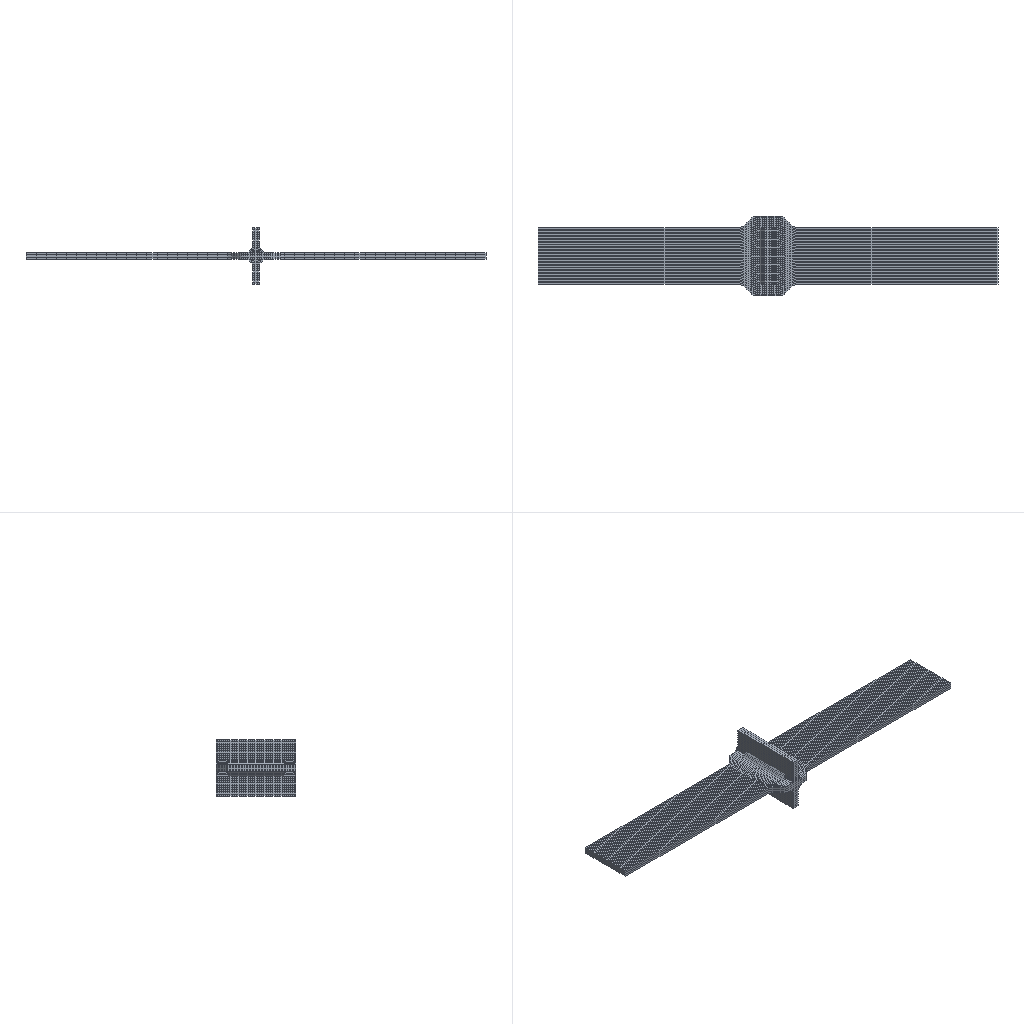Simulation study | abaqus
Set-up summary:
category,name,step,type,value,unit,region
solver,abaqus
solver,version,,,Abaqus/Standard 3DEXPERIENCE R2017x
units,not stated in the deck,,not stated
analysis,deck,,coupled temperature-displacement,coupled temperature-displacement
load_step,Step-del,Step-del,coupled temperature-displacement
load_step,Step-add,Step-add,coupled temperature-displacement
load_step,requested,,,2
mesh,nodes,,,15296
mesh,elements,,,11153
element_type,C3D8RT,,solid,11153
load,load commands in deck,,count,3
bc,support commands in deck,,count,3
material,MATERIAL-1,,in results
check,setup vs results,,match,"per instance, exact: element labels, types and connectivity; labels of the nodes the elements use; coordinates of those nodes at SINGLE_PRECISION in 1 of 2 instance(s)"
Abaqus input file, long lists of numbers shortened:
*Heading
** Job name: Job-1 Model name: Model-1
** Generated by: Abaqus/CAE 2017
*Preprint, echo=NO, model=NO, history=NO, contact=NO
**
** PARTS
**
*Part, name=Part-1
*Node
      1,  -10.243,          70.,           6.
      2,  -10.243,          70.,           0.
** (14566 more lines like these left out)
*Element, type=C3D8RT
1,  134, 1857,  129,    1,  135, 1859,  136,    6
2, 1857, 1858,  130,  129, 1859, 1860,  137,  136
** (10676 more lines like these left out)
*Nset, nset=Set-5, generate
     1,  14568,      1
*Elset, elset=Set-5, generate
     1,  10678,      1
** Section: Section-1
*Solid Section, elset=Set-5, material=Material-1
,
*End Part
**
*Part, name=add
*Node
      1,   4.243,          60.,           6.
      2,   4.243,          10.,           6.
** (726 more lines like these left out)
*Element, type=C3D8RT
  1, 273, 276,  96,  95, 441, 444, 299, 300
  2, 276, 275,  97,  96, 444, 443, 298, 299
** (473 more lines like these left out)
*Nset, nset=Set-5, generate
   1,  728,    1
*Elset, elset=Set-5, generate
   1,  475,    1
** Section: Section-1
*Solid Section, elset=Set-5, material=Material-1
,
*End Part
**
**
** ASSEMBLY
**
*Assembly, name=Assembly
**
*Instance, name=Part-1-1, part=Part-1
    -2.121,         -10.,     -8.121
*End Instance
**
*Instance, name=add-1, part=add
    -2.121,         -10.,     -8.121
*End Instance
**
*Nset, nset=Set-1, instance=Part-1-1
    13,    14,    15,    16,    33,    34,    44,    45,    49,    50,    54,    55,    65,    70,    71,    76
    82,    91,   213,   214,   215,   216,   217,   218,   219,   220,   221,   222,   223,   224,   225,   226
** (52 more lines like these left out)
*Elset, elset=Set-1, instance=Part-1-1, generate
 10213,  10637,      1
*Nset, nset=Set-4, instance=Part-1-1
    99,   100,   103,   104,   109,   110,   111,   112,   115,   116,   119,   120,   125,   126,   127,   128
  1024,  1025,  1026,  1027,  1028,  1029,  1030,  1031,  1032,  1033,  1034,  1035,  1036,  1037,  1038,  1039
** (397 more lines like these left out)
*Elset, elset=Set-4, instance=Part-1-1
 4108, 4109, 4110, 4111, 4112, 4113, 4114, 4115, 4116, 4117, 4118, 4119, 4120, 4121, 4122, 4123
 4124, 4125, 4126, 4127, 4128, 4129, 4130, 4131, 4132, 4133, 4134, 4135, 4136, 4137, 4138, 4139
** (276 more lines like these left out)
*Nset, nset=Set-5, instance=Part-1-1, generate
     1,  14568,      1
*Elset, elset=Set-5, instance=Part-1-1, generate
     1,  10678,      1
*Nset, nset=Set-6, instance=add-1, generate
   1,  728,    1
*Elset, elset=Set-6, instance=add-1, generate
   1,  475,    1
*Nset, nset=Set-7, instance=Part-1-1, generate
     1,  14568,      1
*Nset, nset=Set-7, instance=add-1, generate
   1,  728,    1
*Elset, elset=Set-7, instance=Part-1-1, generate
     1,  10678,      1
*Elset, elset=Set-7, instance=add-1, generate
   1,  475,    1
*Nset, nset=Set-8, instance=Part-1-1
    13,    14,    15,    16,    33,    34,    44,    45,    49,    50,    54,    55,    65,    70,    71,    76
    82,    91,   213,   214,   215,   216,   217,   218,   219,   220,   221,   222,   223,   224,   225,   226
** (52 more lines like these left out)
*Nset, nset=Set-8, instance=add-1, generate
   1,  728,    1
*Elset, elset=Set-8, instance=Part-1-1, generate
 10213,  10637,      1
*Elset, elset=Set-8, instance=add-1, generate
   1,  475,    1
*Nset, nset=Set-9, instance=add-1, generate
   1,  728,    1
*Elset, elset=Set-9, instance=add-1, generate
   1,  475,    1
*Elset, elset=_Surf-1_S4, internal, instance=Part-1-1
     3,     6,     9,    12,    15,    18,    21,    24,    27,    30,    33,    36,    39,    42,    45,    48
    51,    54,    57,    60,    63,    66,    69,    72,    75,    78,    81,    84,    87,    90,    93,    96
** (63 more lines like these left out)
*Elset, elset=_Surf-1_S6, internal, instance=Part-1-1
     1,     4,     7,    10,    13,    16,    19,    22,    25,    28,    31,    34,    37,    40,    43,    46
    49,    52,    55,    58,    61,    64,    67,    70,    73,    76,    79,    82,    85,    88,    91,    94
** (50 more lines like these left out)
*Elset, elset=_Surf-1_S3, internal, instance=Part-1-1
  445,  446,  447,  556,  557,  558,  667,  668,  669,  781,  784,  787,  790,  793,  871,  874
  877,  880,  883,  892,  895,  898,  901,  904,  982,  985,  988,  991,  994, 1003, 1006, 1009
** (38 more lines like these left out)
*Elset, elset=_Surf-1_S5, internal, instance=Part-1-1
   553,   554,   555,   664,   665,   666,   775,   776,   777,   783,   786,   789,   792,   795,   873,   876
   879,   882,   885,   894,   897,   900,   903,   906,   984,   987,   990,   993,   996,  1005,  1008,  1011
** (31 more lines like these left out)
*Elset, elset=_Surf-1_S1, internal, instance=Part-1-1
     1,     2,     3,     4,     5,     6,   223,   224,   225,   226,   227,   228,  3553,  3554,  3555,  3556
  3557,  3558,  3559,  3560,  3561,  3562,  3563,  3564,  3565,  3566,  3567,  3568,  3569,  3570,  3571,  3572
** (133 more lines like these left out)
*Elset, elset=_Surf-1_S2, internal, instance=Part-1-1
   217,   218,   219,   220,   221,   222,   439,   440,   441,   442,   443,   444,  1999,  2000,  2001,  2002
  2003,  2004,  2005,  2006,  2007,  2008,  2009,  2010,  2011,  2012,  2013,  2014,  2015,  2016,  2017,  2018
** (147 more lines like these left out)
*Surface, type=ELEMENT, name=Surf-1
_Surf-1_S4, S4
_Surf-1_S6, S6
_Surf-1_S2, S2
_Surf-1_S3, S3
_Surf-1_S5, S5
_Surf-1_S1, S1
*Elset, elset=_Surf-2_S4, internal, instance=Part-1-1
     3,     6,     9,    12,    15,    18,    21,    24,    27,    30,    33,    36,    39,    42,    45,    48
    51,    54,    57,    60,    63,    66,    69,    72,    75,    78,    81,    84,    87,    90,    93,    96
** (63 more lines like these left out)
*Elset, elset=_Surf-2_S6, internal, instance=Part-1-1
     1,     4,     7,    10,    13,    16,    19,    22,    25,    28,    31,    34,    37,    40,    43,    46
    49,    52,    55,    58,    61,    64,    67,    70,    73,    76,    79,    82,    85,    88,    91,    94
** (50 more lines like these left out)
*Elset, elset=_Surf-2_S3, internal, instance=Part-1-1
  445,  446,  447,  556,  557,  558,  667,  668,  669,  781,  784,  787,  790,  793,  871,  874
  877,  880,  883,  892,  895,  898,  901,  904,  982,  985,  988,  991,  994, 1003, 1006, 1009
** (38 more lines like these left out)
*Elset, elset=_Surf-2_S5, internal, instance=Part-1-1
   553,   554,   555,   664,   665,   666,   775,   776,   777,   783,   786,   789,   792,   795,   873,   876
   879,   882,   885,   894,   897,   900,   903,   906,   984,   987,   990,   993,   996,  1005,  1008,  1011
** (31 more lines like these left out)
*Elset, elset=_Surf-2_S1, internal, instance=Part-1-1
     1,     2,     3,     4,     5,     6,   223,   224,   225,   226,   227,   228,  3553,  3554,  3555,  3556
  3557,  3558,  3559,  3560,  3561,  3562,  3563,  3564,  3565,  3566,  3567,  3568,  3569,  3570,  3571,  3572
** (133 more lines like these left out)
*Elset, elset=_Surf-2_S2, internal, instance=Part-1-1
   217,   218,   219,   220,   221,   222,   439,   440,   441,   442,   443,   444,  1999,  2000,  2001,  2002
  2003,  2004,  2005,  2006,  2007,  2008,  2009,  2010,  2011,  2012,  2013,  2014,  2015,  2016,  2017,  2018
** (147 more lines like these left out)
*Surface, type=ELEMENT, name=Surf-2
_Surf-2_S4, S4
_Surf-2_S6, S6
_Surf-2_S2, S2
_Surf-2_S3, S3
_Surf-2_S5, S5
_Surf-2_S1, S1
*Elset, elset=_Surf-5_S4, internal, instance=Part-1-1
     3,     6,     9,    12,    15,    18,    21,    24,    27,    30,    33,    36,    39,    42,    45,    48
    51,    54,    57,    60,    63,    66,    69,    72,    75,    78,    81,    84,    87,    90,    93,    96
** (63 more lines like these left out)
*Elset, elset=_Surf-5_S4, internal, instance=add-1
   4,   7,  10,  13,  16,  17,  18,  19,  23,  26,  29,  32,  35,  36,  37,  38
  42,  45,  48,  51,  54,  55,  56,  57,  61,  64,  67,  70,  73,  74,  75,  76
** (11 more lines like these left out)
*Elset, elset=_Surf-5_S6, internal, instance=Part-1-1
     1,     4,     7,    10,    13,    16,    19,    22,    25,    28,    31,    34,    37,    40,    43,    46
    49,    52,    55,    58,    61,    64,    67,    70,    73,    76,    79,    82,    85,    88,    91,    94
** (50 more lines like these left out)
*Elset, elset=_Surf-5_S3, internal, instance=Part-1-1
  445,  446,  447,  556,  557,  558,  667,  668,  669,  781,  784,  787,  790,  793,  871,  874
  877,  880,  883,  892,  895,  898,  901,  904,  982,  985,  988,  991,  994, 1003, 1006, 1009
** (38 more lines like these left out)
*Elset, elset=_Surf-5_S5, internal, instance=Part-1-1
   553,   554,   555,   664,   665,   666,   775,   776,   777,   783,   786,   789,   792,   795,   873,   876
   879,   882,   885,   894,   897,   900,   903,   906,   984,   987,   990,   993,   996,  1005,  1008,  1011
** (31 more lines like these left out)
*Elset, elset=_Surf-5_S5, internal, instance=add-1
   1,   2,   3,   4,   5,   6,   7,  17,  20,  21,  22,  23,  24,  25,  26,  36
  39,  40,  41,  42,  43,  44,  45,  55,  58,  59,  60,  61,  62,  63,  64,  74
** (11 more lines like these left out)
*Elset, elset=_Surf-5_S1, internal, instance=Part-1-1
     1,     2,     3,     4,     5,     6,   223,   224,   225,   226,   227,   228,  3553,  3554,  3555,  3556
  3557,  3558,  3559,  3560,  3561,  3562,  3563,  3564,  3565,  3566,  3567,  3568,  3569,  3570,  3571,  3572
** (133 more lines like these left out)
*Elset, elset=_Surf-5_S1, internal, instance=add-1, generate
  1,  19,   1
*Elset, elset=_Surf-5_S2, internal, instance=Part-1-1
   217,   218,   219,   220,   221,   222,   439,   440,   441,   442,   443,   444,  1999,  2000,  2001,  2002
  2003,  2004,  2005,  2006,  2007,  2008,  2009,  2010,  2011,  2012,  2013,  2014,  2015,  2016,  2017,  2018
** (147 more lines like these left out)
*Elset, elset=_Surf-5_S2, internal, instance=add-1, generate
 457,  475,    1
*Surface, type=ELEMENT, name=Surf-5
_Surf-5_S4, S4
_Surf-5_S6, S6
_Surf-5_S2, S2
_Surf-5_S3, S3
_Surf-5_S5, S5
_Surf-5_S1, S1
*Elset, elset=_Surf-6_S4, internal, instance=Part-1-1
     3,     6,     9,    12,    15,    18,    21,    24,    27,    30,    33,    36,    39,    42,    45,    48
    51,    54,    57,    60,    63,    66,    69,    72,    75,    78,    81,    84,    87,    90,    93,    96
** (63 more lines like these left out)
*Elset, elset=_Surf-6_S4, internal, instance=add-1
   4,   7,  10,  13,  16,  17,  18,  19,  23,  26,  29,  32,  35,  36,  37,  38
  42,  45,  48,  51,  54,  55,  56,  57,  61,  64,  67,  70,  73,  74,  75,  76
** (11 more lines like these left out)
*Elset, elset=_Surf-6_S6, internal, instance=Part-1-1
     1,     4,     7,    10,    13,    16,    19,    22,    25,    28,    31,    34,    37,    40,    43,    46
    49,    52,    55,    58,    61,    64,    67,    70,    73,    76,    79,    82,    85,    88,    91,    94
** (50 more lines like these left out)
*Elset, elset=_Surf-6_S3, internal, instance=Part-1-1
  445,  446,  447,  556,  557,  558,  667,  668,  669,  781,  784,  787,  790,  793,  871,  874
  877,  880,  883,  892,  895,  898,  901,  904,  982,  985,  988,  991,  994, 1003, 1006, 1009
** (38 more lines like these left out)
*Elset, elset=_Surf-6_S5, internal, instance=Part-1-1
   553,   554,   555,   664,   665,   666,   775,   776,   777,   783,   786,   789,   792,   795,   873,   876
   879,   882,   885,   894,   897,   900,   903,   906,   984,   987,   990,   993,   996,  1005,  1008,  1011
** (31 more lines like these left out)
*Elset, elset=_Surf-6_S5, internal, instance=add-1
   1,   2,   3,   4,   5,   6,   7,  17,  20,  21,  22,  23,  24,  25,  26,  36
  39,  40,  41,  42,  43,  44,  45,  55,  58,  59,  60,  61,  62,  63,  64,  74
** (11 more lines like these left out)
*Elset, elset=_Surf-6_S1, internal, instance=Part-1-1
     1,     2,     3,     4,     5,     6,   223,   224,   225,   226,   227,   228,  3553,  3554,  3555,  3556
  3557,  3558,  3559,  3560,  3561,  3562,  3563,  3564,  3565,  3566,  3567,  3568,  3569,  3570,  3571,  3572
** (133 more lines like these left out)
*Elset, elset=_Surf-6_S1, internal, instance=add-1, generate
  1,  19,   1
*Elset, elset=_Surf-6_S2, internal, instance=Part-1-1
   217,   218,   219,   220,   221,   222,   439,   440,   441,   442,   443,   444,  1999,  2000,  2001,  2002
  2003,  2004,  2005,  2006,  2007,  2008,  2009,  2010,  2011,  2012,  2013,  2014,  2015,  2016,  2017,  2018
** (147 more lines like these left out)
*Elset, elset=_Surf-6_S2, internal, instance=add-1, generate
 457,  475,    1
*Surface, type=ELEMENT, name=Surf-6
_Surf-6_S4, S4
_Surf-6_S6, S6
_Surf-6_S2, S2
_Surf-6_S3, S3
_Surf-6_S5, S5
_Surf-6_S1, S1
*Elset, elset=_m_Surf-3_S4, internal, instance=add-1
   4,   7,  10,  13,  16,  23,  26,  29,  32,  35,  42,  45,  48,  51,  54,  61
  64,  67,  70,  73,  80,  83,  86,  89,  92,  99, 102, 105, 108, 111, 118, 121
** (6 more lines like these left out)
*Elset, elset=_m_Surf-3_S5, internal, instance=add-1
   5,   6,   7,  17,  24,  25,  26,  36,  43,  44,  45,  55,  62,  63,  64,  74
  81,  82,  83,  93, 100, 101, 102, 112, 119, 120, 121, 131, 138, 139, 140, 150
** (5 more lines like these left out)
*Surface, type=ELEMENT, name=m_Surf-3
_m_Surf-3_S4, S4
_m_Surf-3_S5, S5
*Elset, elset=_s_Surf-3_S4, internal, instance=Part-1-1
 2115, 2118, 2121, 2124, 2127, 2130, 2133, 2136, 2139, 2142, 2145, 2148, 2151, 2154, 2157, 2160
 2163, 2166, 2169, 2172, 2175, 2178, 2181, 2184, 2187, 2190, 2193, 2196, 2199, 2202, 2205, 2208
** (7 more lines like these left out)
*Elset, elset=_s_Surf-3_S6, internal, instance=Part-1-1, generate
 3886,  4099,     3
*Surface, type=ELEMENT, name=s_Surf-3
_s_Surf-3_S4, S4
_s_Surf-3_S6, S6
** Constraint: Constraint-1
*Tie, name=Constraint-1, adjust=yes
s_Surf-3, m_Surf-3
*End Assembly
**
** MATERIALS
**
*Material, name=Material-1
*Conductivity
45.,
*Density
 7.8e-09,
*Elastic
210000., 0.3
*Expansion
 1.2e-05,
*Plastic
350.,0.
*Specific Heat
 4.6e+08,
**
** PHYSICAL CONSTANTS
**
*Physical Constants, absolute zero=-273., stefan boltzmann=5.67e-08
**
** PREDEFINED FIELDS
**
** Name: Predefined Field-1   Type: Temperature
*Initial Conditions, type=TEMPERATURE
Set-7, 20.
** ----------------------------------------------------------------
**
** STEP: Step-del
**
*Step, name=Step-del, nlgeom=NO
*Coupled Temperature-displacement, creep=none, deltmx=1e+12, stabilize=0.0002, allsdtol=0.05, continue=NO
0.0001, 0.0001, 1e-09, 0.0001
**
** BOUNDARY CONDITIONS
**
** Name: BC-1 Type: 对称/反对称/完全固定
*Boundary
Set-4, ENCASTRE
**
** INTERACTIONS
**
** Interaction: Int-del
*Model Change, remove
Set-8,
**
** OUTPUT REQUESTS
**
*Restart, write, frequency=0
**
** FIELD OUTPUT: F-Output-1
**
*Output, field
*Node Output
CF, NT, RF, RFL, RM, RT, U, V
*Element Output, directions=YES
E, HFL, LE, MISES, MISESMAX, MISESONLY, PE, PEEQ, PEEQMAX, PEEQT, PEMAG, S, SSAVG, TEMP
*Contact Output
CDISP, CSTRESS
*Radiation Output
FTEMP,
**
** HISTORY OUTPUT: H-Output-1
**
*Output, history, variable=PRESELECT
*End Step
** ----------------------------------------------------------------
**
** STEP: Step-add
**
*Step, name=Step-add, nlgeom=YES, inc=10000000
*Coupled Temperature-displacement, creep=none, deltmx=1e+12, stabilize=0.0002, allsdtol=0.05, continue=NO
0.05, 10., 1e-05, 0.5
**
** LOADS
**
** Name: Load-1   Type: Body heat flux
*Dflux
Set-6, BFNU, 1.
**
** INTERACTIONS
**
** Interaction: Int-add
*Model Change, add
Set-9,
** Interaction: Int-3
*Sradiate
Surf-5, R, 20., 0.5
** Interaction: Int-4
*Sfilm
Surf-6, F, 20., 0.001
**
** OUTPUT REQUESTS
**
*Restart, write, frequency=0
**
** FIELD OUTPUT: F-Output-1
**
*Output, field
*Node Output
CF, NT, RF, RFL, RM, RT, U, V
*Element Output, directions=YES
E, HFL, LE, MISES, MISESMAX, MISESONLY, PE, PEEQ, PEEQMAX, PEEQT, PEMAG, S, SSAVG, TEMP
*Contact Output
CDISP, CSTRESS
*Radiation Output
FTEMP,
**
** HISTORY OUTPUT: H-Output-1
**
*Output, history, variable=PRESELECT
*End Step
Results summary:
result,step,,completed,increments=1 time=0.0001/0.0001
result,step,,completed,increments=51 time=10.0/10.0
result,analysis,,,"coupled temperature-displacement, steady state"
result,last_loadstep,,,2
result,primary field,,,"U, NT11"
result,reaction total,,FX,0.6884,model units
result,reaction total,,FY,0.6371,model units
result,reaction total,,FZ,-2.875,model units